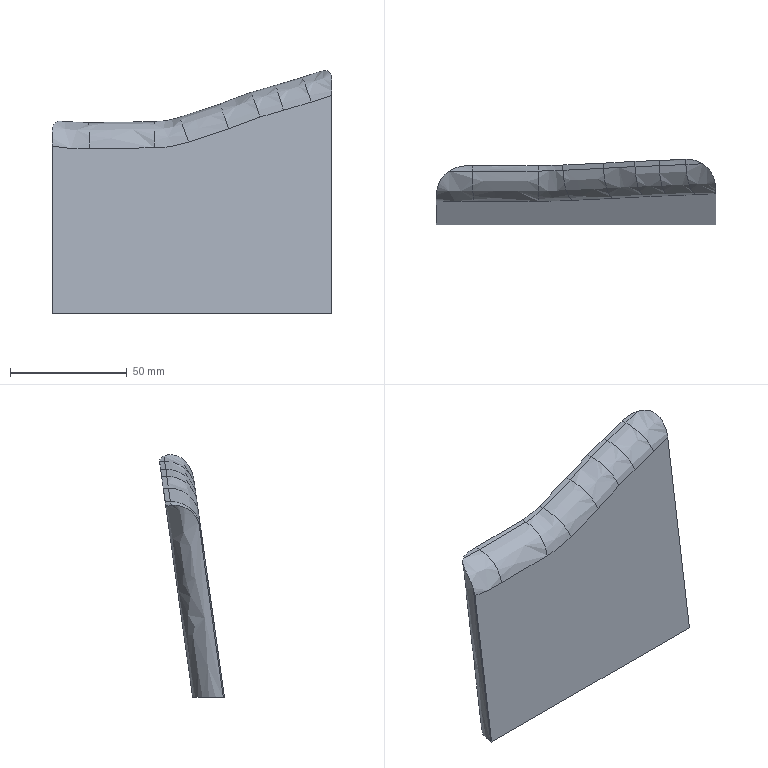Part | STEP file | solid 58 | 1 solid | 23 faces | box 120 x 27.859 x 104.131 mm | volume 135753 mm3 | spline 12 | other 8 | plane 3